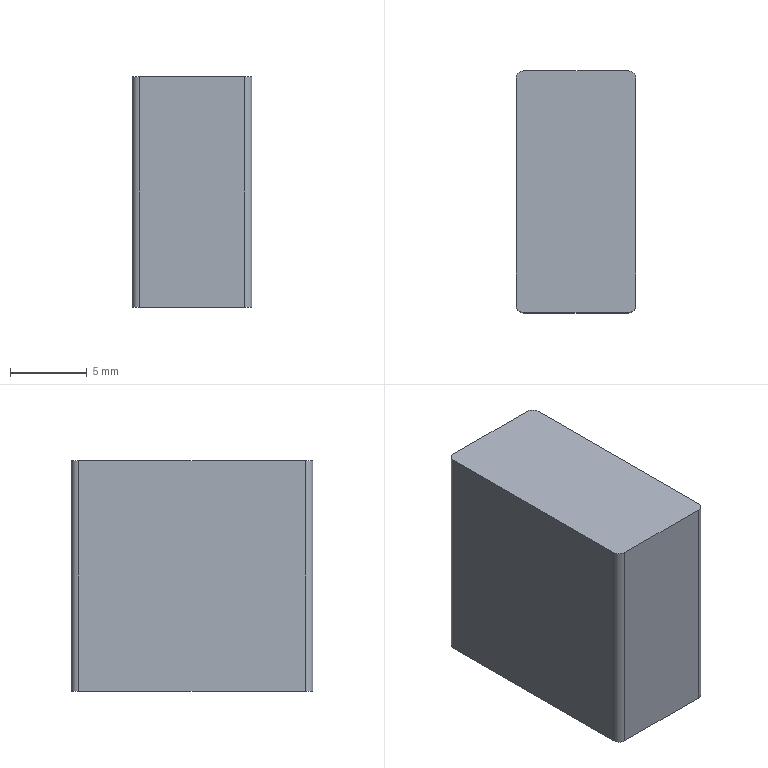Part | NX | features BREP 1 | 1 solid | 10 faces | box 7.8 x 15.754 x 15 mm | volume 1840 mm3 | plane 6 | cylinder 4 | commonest cylinder face diameters 1 x4
STEP:
#1=CARTESIAN_POINT('',(-3.4,7.877,-25.6));
#2=VERTEX_POINT('',#1);
#3=CARTESIAN_POINT('',(-3.9,7.377,-25.6));
#4=VERTEX_POINT('',#3);
#5=CARTESIAN_POINT('',(-3.4,7.377,-25.6));
#6=DIRECTION('',(0.,0.,1.));
#7=DIRECTION('',(1.,0.,0.));
#8=AXIS2_PLACEMENT_3D('',#5,#6,#7);
#9=CIRCLE('',#8,0.5);
#10=EDGE_CURVE('',#2,#4,#9,.T.);
#11=ORIENTED_EDGE('',*,*,#10,.F.);
#12=CARTESIAN_POINT('',(-3.4,7.877,-40.6));
#13=VERTEX_POINT('',#12);
#14=CARTESIAN_POINT('',(-3.4,7.877,-40.6));
#15=DIRECTION('',(0.,0.,1.));
#16=VECTOR('',#15,1000.);
#17=LINE('',#14,#16);
#18=EDGE_CURVE('',#13,#2,#17,.T.);
#19=ORIENTED_EDGE('',*,*,#18,.F.);
#20=CARTESIAN_POINT('',(-3.9,7.377,-40.6));
#21=VERTEX_POINT('',#20);
#22=CARTESIAN_POINT('',(-3.4,7.377,-40.6));
#23=DIRECTION('',(0.,0.,1.));
#24=DIRECTION('',(1.,0.,0.));
#25=AXIS2_PLACEMENT_3D('',#22,#23,#24);
#26=CIRCLE('',#25,0.5);
#27=EDGE_CURVE('',#13,#21,#26,.T.);
#28=ORIENTED_EDGE('',*,*,#27,.T.);
#29=CARTESIAN_POINT('',(-3.9,7.377,-40.6));
#30=DIRECTION('',(0.,0.,1.));
#31=VECTOR('',#30,1000.);
#32=LINE('',#29,#31);
#33=EDGE_CURVE('',#21,#4,#32,.T.);
#34=ORIENTED_EDGE('',*,*,#33,.T.);
#35=EDGE_LOOP('',(#11,#19,#28,#34));
#36=FACE_BOUND('',#35,.T.);
#37=CARTESIAN_POINT('',(-3.4,7.377,-40.6));
#38=DIRECTION('',(0.,0.,1.));
#39=DIRECTION('',(-1.,0.,0.));
#40=AXIS2_PLACEMENT_3D('',#37,#38,#39);
#41=CYLINDRICAL_SURFACE('',#40,0.5);
#42=ADVANCED_FACE('',(#36),#41,.T.);
#43=CARTESIAN_POINT('',(-3.9,-7.377,-25.6));
#44=VERTEX_POINT('',#43);
#45=CARTESIAN_POINT('',(-3.9,-7.377,-25.6));
#46=DIRECTION('',(0.,1.,0.));
#47=VECTOR('',#46,1000.);
#48=LINE('',#45,#47);
#49=EDGE_CURVE('',#44,#4,#48,.T.);
#50=ORIENTED_EDGE('',*,*,#49,.T.);
#51=ORIENTED_EDGE('',*,*,#33,.F.);
#52=CARTESIAN_POINT('',(-3.9,-7.377,-40.6));
#53=VERTEX_POINT('',#52);
#54=CARTESIAN_POINT('',(-3.9,-7.377,-40.6));
#55=DIRECTION('',(0.,1.,0.));
#56=VECTOR('',#55,1000.);
#57=LINE('',#54,#56);
#58=EDGE_CURVE('',#53,#21,#57,.T.);
#59=ORIENTED_EDGE('',*,*,#58,.F.);
#60=CARTESIAN_POINT('',(-3.9,-7.377,-40.6));
#61=DIRECTION('',(0.,0.,1.));
#62=VECTOR('',#61,1000.);
#63=LINE('',#60,#62);
#64=EDGE_CURVE('',#53,#44,#63,.T.);
#65=ORIENTED_EDGE('',*,*,#64,.T.);
#66=EDGE_LOOP('',(#50,#51,#59,#65));
#67=FACE_BOUND('',#66,.T.);
#68=CARTESIAN_POINT('',(-3.9,-7.377,-40.6));
#69=DIRECTION('',(1.,0.,0.));
#70=DIRECTION('',(0.,0.,1.));
#71=AXIS2_PLACEMENT_3D('',#68,#69,#70);
#72=PLANE('',#71);
#73=ADVANCED_FACE('',(#67),#72,.F.);
#74=CARTESIAN_POINT('',(-3.4,-7.877,-25.6));
#75=VERTEX_POINT('',#74);
#76=CARTESIAN_POINT('',(-3.4,-7.377,-25.6));
#77=DIRECTION('',(0.,0.,1.));
#78=DIRECTION('',(1.,0.,0.));
#79=AXIS2_PLACEMENT_3D('',#76,#77,#78);
#80=CIRCLE('',#79,0.5);
#81=EDGE_CURVE('',#44,#75,#80,.T.);
#82=ORIENTED_EDGE('',*,*,#81,.F.);
#83=ORIENTED_EDGE('',*,*,#64,.F.);
#84=CARTESIAN_POINT('',(-3.4,-7.877,-40.6));
#85=VERTEX_POINT('',#84);
#86=CARTESIAN_POINT('',(-3.4,-7.377,-40.6));
#87=DIRECTION('',(0.,0.,1.));
#88=DIRECTION('',(1.,0.,0.));
#89=AXIS2_PLACEMENT_3D('',#86,#87,#88);
#90=CIRCLE('',#89,0.5);
#91=EDGE_CURVE('',#53,#85,#90,.T.);
#92=ORIENTED_EDGE('',*,*,#91,.T.);
#93=CARTESIAN_POINT('',(-3.4,-7.877,-40.6));
#94=DIRECTION('',(0.,0.,1.));
#95=VECTOR('',#94,1000.);
#96=LINE('',#93,#95);
#97=EDGE_CURVE('',#85,#75,#96,.T.);
#98=ORIENTED_EDGE('',*,*,#97,.T.);
#99=EDGE_LOOP('',(#82,#83,#92,#98));
#100=FACE_BOUND('',#99,.T.);
#101=CARTESIAN_POINT('',(-3.4,-7.377,-40.6));
#102=DIRECTION('',(0.,0.,1.));
#103=DIRECTION('',(-1.,0.,0.));
#104=AXIS2_PLACEMENT_3D('',#101,#102,#103);
#105=CYLINDRICAL_SURFACE('',#104,0.5);
#106=ADVANCED_FACE('',(#100),#105,.T.);
#107=CARTESIAN_POINT('',(3.4,-7.877,-25.6));
#108=VERTEX_POINT('',#107);
#109=CARTESIAN_POINT('',(3.4,-7.877,-25.6));
#110=DIRECTION('',(-1.,0.,0.));
#111=VECTOR('',#110,1000.);
#112=LINE('',#109,#111);
#113=EDGE_CURVE('',#108,#75,#112,.T.);
#114=ORIENTED_EDGE('',*,*,#113,.T.);
#115=ORIENTED_EDGE('',*,*,#97,.F.);
#116=CARTESIAN_POINT('',(3.4,-7.877,-40.6));
#117=VERTEX_POINT('',#116);
#118=CARTESIAN_POINT('',(3.4,-7.877,-40.6));
#119=DIRECTION('',(-1.,0.,0.));
#120=VECTOR('',#119,1000.);
#121=LINE('',#118,#120);
#122=EDGE_CURVE('',#117,#85,#121,.T.);
#123=ORIENTED_EDGE('',*,*,#122,.F.);
#124=CARTESIAN_POINT('',(3.4,-7.877,-40.6));
#125=DIRECTION('',(0.,0.,1.));
#126=VECTOR('',#125,1000.);
#127=LINE('',#124,#126);
#128=EDGE_CURVE('',#117,#108,#127,.T.);
#129=ORIENTED_EDGE('',*,*,#128,.T.);
#130=EDGE_LOOP('',(#114,#115,#123,#129));
#131=FACE_BOUND('',#130,.T.);
#132=CARTESIAN_POINT('',(3.4,-7.877,-40.6));
#133=DIRECTION('',(0.,1.,0.));
#134=DIRECTION('',(0.,0.,-1.));
#135=AXIS2_PLACEMENT_3D('',#132,#133,#134);
#136=PLANE('',#135);
#137=ADVANCED_FACE('',(#131),#136,.F.);
#138=CARTESIAN_POINT('',(3.9,-7.377,-25.6));
#139=VERTEX_POINT('',#138);
#140=CARTESIAN_POINT('',(3.4,-7.377,-25.6));
#141=DIRECTION('',(0.,0.,1.));
#142=DIRECTION('',(1.,0.,0.));
#143=AXIS2_PLACEMENT_3D('',#140,#141,#142);
#144=CIRCLE('',#143,0.5);
#145=EDGE_CURVE('',#108,#139,#144,.T.);
#146=ORIENTED_EDGE('',*,*,#145,.F.);
#147=ORIENTED_EDGE('',*,*,#128,.F.);
#148=CARTESIAN_POINT('',(3.9,-7.377,-40.6));
#149=VERTEX_POINT('',#148);
#150=CARTESIAN_POINT('',(3.4,-7.377,-40.6));
#151=DIRECTION('',(0.,0.,1.));
#152=DIRECTION('',(1.,0.,0.));
#153=AXIS2_PLACEMENT_3D('',#150,#151,#152);
#154=CIRCLE('',#153,0.5);
#155=EDGE_CURVE('',#117,#149,#154,.T.);
#156=ORIENTED_EDGE('',*,*,#155,.T.);
#157=CARTESIAN_POINT('',(3.9,-7.377,-40.6));
#158=DIRECTION('',(0.,0.,1.));
#159=VECTOR('',#158,1000.);
#160=LINE('',#157,#159);
#161=EDGE_CURVE('',#149,#139,#160,.T.);
#162=ORIENTED_EDGE('',*,*,#161,.T.);
#163=EDGE_LOOP('',(#146,#147,#156,#162));
#164=FACE_BOUND('',#163,.T.);
#165=CARTESIAN_POINT('',(3.4,-7.377,-40.6));
#166=DIRECTION('',(0.,0.,1.));
#167=DIRECTION('',(-1.,0.,0.));
#168=AXIS2_PLACEMENT_3D('',#165,#166,#167);
#169=CYLINDRICAL_SURFACE('',#168,0.5);
#170=ADVANCED_FACE('',(#164),#169,.T.);
#171=CARTESIAN_POINT('',(3.9,7.377,-25.6));
#172=VERTEX_POINT('',#171);
#173=CARTESIAN_POINT('',(3.9,7.377,-25.6));
#174=DIRECTION('',(0.,-1.,0.));
#175=VECTOR('',#174,1000.);
#176=LINE('',#173,#175);
#177=EDGE_CURVE('',#172,#139,#176,.T.);
#178=ORIENTED_EDGE('',*,*,#177,.T.);
#179=ORIENTED_EDGE('',*,*,#161,.F.);
#180=CARTESIAN_POINT('',(3.9,7.377,-40.6));
#181=VERTEX_POINT('',#180);
#182=CARTESIAN_POINT('',(3.9,7.377,-40.6));
#183=DIRECTION('',(0.,-1.,0.));
#184=VECTOR('',#183,1000.);
#185=LINE('',#182,#184);
#186=EDGE_CURVE('',#181,#149,#185,.T.);
#187=ORIENTED_EDGE('',*,*,#186,.F.);
#188=CARTESIAN_POINT('',(3.9,7.377,-40.6));
#189=DIRECTION('',(0.,0.,1.));
#190=VECTOR('',#189,1000.);
#191=LINE('',#188,#190);
#192=EDGE_CURVE('',#181,#172,#191,.T.);
#193=ORIENTED_EDGE('',*,*,#192,.T.);
#194=EDGE_LOOP('',(#178,#179,#187,#193));
#195=FACE_BOUND('',#194,.T.);
#196=CARTESIAN_POINT('',(3.9,7.377,-40.6));
#197=DIRECTION('',(-1.,0.,0.));
#198=DIRECTION('',(0.,1.,0.));
#199=AXIS2_PLACEMENT_3D('',#196,#197,#198);
#200=PLANE('',#199);
#201=ADVANCED_FACE('',(#195),#200,.F.);
#202=CARTESIAN_POINT('',(3.4,7.877,-25.6));
#203=VERTEX_POINT('',#202);
#204=CARTESIAN_POINT('',(3.4,7.377,-25.6));
#205=DIRECTION('',(0.,0.,1.));
#206=DIRECTION('',(1.,0.,0.));
#207=AXIS2_PLACEMENT_3D('',#204,#205,#206);
#208=CIRCLE('',#207,0.5);
#209=EDGE_CURVE('',#172,#203,#208,.T.);
#210=ORIENTED_EDGE('',*,*,#209,.F.);
#211=ORIENTED_EDGE('',*,*,#192,.F.);
#212=CARTESIAN_POINT('',(3.4,7.877,-40.6));
#213=VERTEX_POINT('',#212);
#214=CARTESIAN_POINT('',(3.4,7.377,-40.6));
#215=DIRECTION('',(0.,0.,1.));
#216=DIRECTION('',(1.,0.,0.));
#217=AXIS2_PLACEMENT_3D('',#214,#215,#216);
#218=CIRCLE('',#217,0.5);
#219=EDGE_CURVE('',#181,#213,#218,.T.);
#220=ORIENTED_EDGE('',*,*,#219,.T.);
#221=CARTESIAN_POINT('',(3.4,7.877,-40.6));
#222=DIRECTION('',(0.,0.,1.));
#223=VECTOR('',#222,1000.);
#224=LINE('',#221,#223);
#225=EDGE_CURVE('',#213,#203,#224,.T.);
#226=ORIENTED_EDGE('',*,*,#225,.T.);
#227=EDGE_LOOP('',(#210,#211,#220,#226));
#228=FACE_BOUND('',#227,.T.);
#229=CARTESIAN_POINT('',(3.4,7.377,-40.6));
#230=DIRECTION('',(0.,0.,1.));
#231=DIRECTION('',(-1.,0.,0.));
#232=AXIS2_PLACEMENT_3D('',#229,#230,#231);
#233=CYLINDRICAL_SURFACE('',#232,0.5);
#234=ADVANCED_FACE('',(#228),#233,.T.);
#235=CARTESIAN_POINT('',(-3.4,7.877,-25.6));
#236=DIRECTION('',(1.,0.,0.));
#237=VECTOR('',#236,1000.);
#238=LINE('',#235,#237);
#239=EDGE_CURVE('',#2,#203,#238,.T.);
#240=ORIENTED_EDGE('',*,*,#239,.T.);
#241=ORIENTED_EDGE('',*,*,#225,.F.);
#242=CARTESIAN_POINT('',(-3.4,7.877,-40.6));
#243=DIRECTION('',(1.,0.,0.));
#244=VECTOR('',#243,1000.);
#245=LINE('',#242,#244);
#246=EDGE_CURVE('',#13,#213,#245,.T.);
#247=ORIENTED_EDGE('',*,*,#246,.F.);
#248=ORIENTED_EDGE('',*,*,#18,.T.);
#249=EDGE_LOOP('',(#240,#241,#247,#248));
#250=FACE_BOUND('',#249,.T.);
#251=CARTESIAN_POINT('',(-3.4,7.877,-40.6));
#252=DIRECTION('',(0.,-1.,0.));
#253=DIRECTION('',(0.,0.,1.));
#254=AXIS2_PLACEMENT_3D('',#251,#252,#253);
#255=PLANE('',#254);
#256=ADVANCED_FACE('',(#250),#255,.F.);
#257=ORIENTED_EDGE('',*,*,#27,.F.);
#258=ORIENTED_EDGE('',*,*,#246,.T.);
#259=ORIENTED_EDGE('',*,*,#219,.F.);
#260=ORIENTED_EDGE('',*,*,#186,.T.);
#261=ORIENTED_EDGE('',*,*,#155,.F.);
#262=ORIENTED_EDGE('',*,*,#122,.T.);
#263=ORIENTED_EDGE('',*,*,#91,.F.);
#264=ORIENTED_EDGE('',*,*,#58,.T.);
#265=EDGE_LOOP('',(#257,#258,#259,#260,#261,#262,#263,#264));
#266=FACE_BOUND('',#265,.T.);
#267=CARTESIAN_POINT('',(-3.4,7.377,-40.6));
#268=DIRECTION('',(0.,0.,1.));
#269=DIRECTION('',(-1.,0.,0.));
#270=AXIS2_PLACEMENT_3D('',#267,#268,#269);
#271=PLANE('',#270);
#272=ADVANCED_FACE('',(#266),#271,.F.);
#273=ORIENTED_EDGE('',*,*,#10,.T.);
#274=ORIENTED_EDGE('',*,*,#49,.F.);
#275=ORIENTED_EDGE('',*,*,#81,.T.);
#276=ORIENTED_EDGE('',*,*,#113,.F.);
#277=ORIENTED_EDGE('',*,*,#145,.T.);
#278=ORIENTED_EDGE('',*,*,#177,.F.);
#279=ORIENTED_EDGE('',*,*,#209,.T.);
#280=ORIENTED_EDGE('',*,*,#239,.F.);
#281=EDGE_LOOP('',(#273,#274,#275,#276,#277,#278,#279,#280));
#282=FACE_BOUND('',#281,.T.);
#283=CARTESIAN_POINT('',(-3.4,7.377,-25.6));
#284=DIRECTION('',(0.,0.,1.));
#285=DIRECTION('',(-1.,0.,0.));
#286=AXIS2_PLACEMENT_3D('',#283,#284,#285);
#287=PLANE('',#286);
#288=ADVANCED_FACE('',(#282),#287,.T.);
#289=CLOSED_SHELL('',(#42,#73,#106,#137,#170,#201,#234,#256,#272,#288));
#290=MANIFOLD_SOLID_BREP('',#289);
#291=(LENGTH_UNIT()NAMED_UNIT(*)SI_UNIT(.MILLI.,.METRE.));
#292=UNCERTAINTY_MEASURE_WITH_UNIT(LENGTH_MEASURE(0.00001),#291,'','');
#293=(NAMED_UNIT(*)PLANE_ANGLE_UNIT()SI_UNIT($,.RADIAN.));
#294=(NAMED_UNIT(*)SI_UNIT($,.STERADIAN.)SOLID_ANGLE_UNIT());
#295=(GEOMETRIC_REPRESENTATION_CONTEXT(3)GLOBAL_UNCERTAINTY_ASSIGNED_CONTEXT((#292))GLOBAL_UNIT_ASSIGNED_CONTEXT((#291,#293,#294))REPRESENTATION_CONTEXT('',''));
#296=ADVANCED_BREP_SHAPE_REPRESENTATION('',(#290),#295);